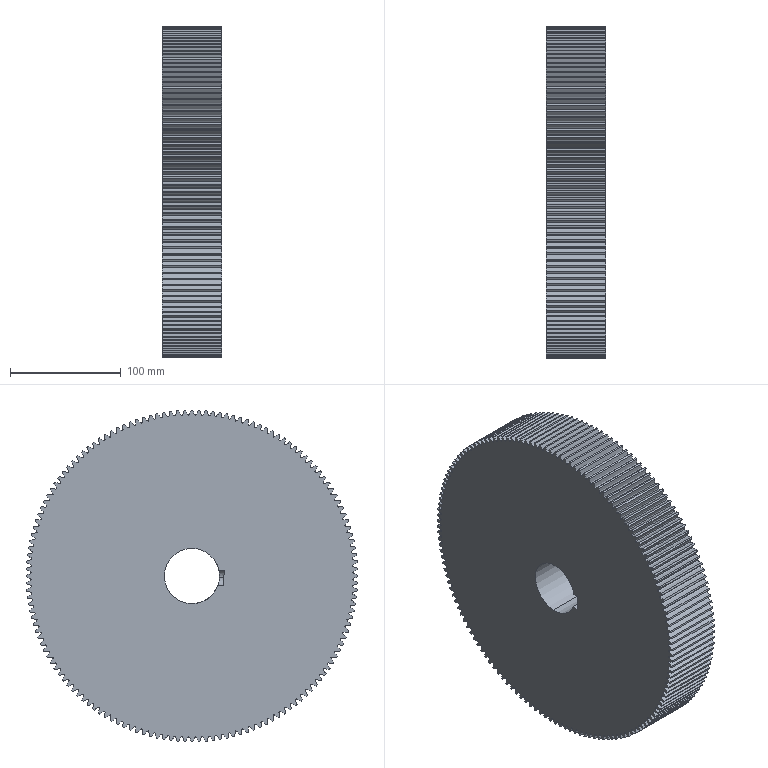Part | STEP file | Cut-Extrude 3-7 | 1 solid | 601 faces | box 54 x 300 x 300 mm | volume 3603686 mm3 | cylinder 300 | spline 296 | plane 5 | commonest cylinder face diameters 291 x148 300 x148 14 x2 50 x2